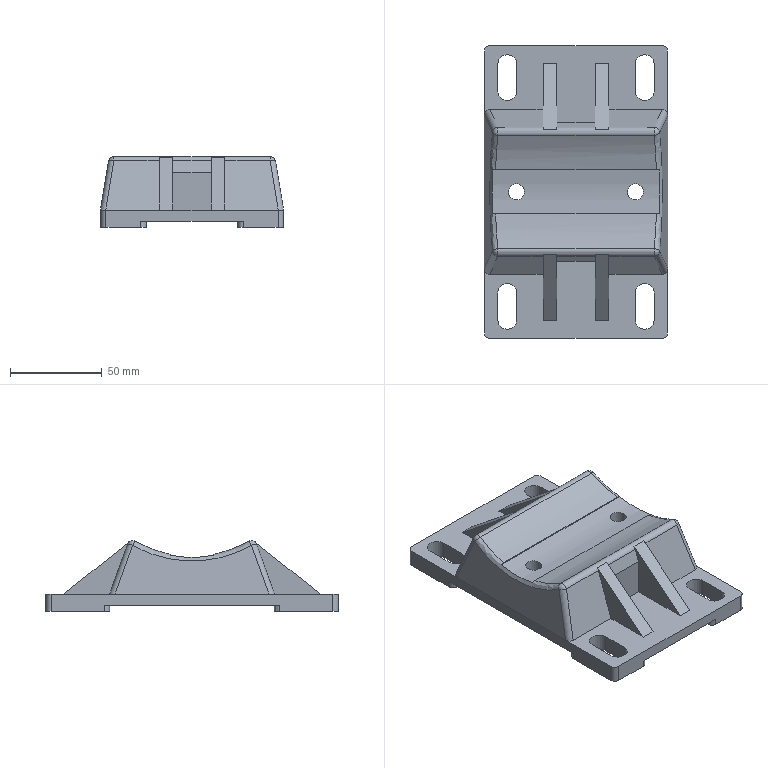Part | STEP file | MDZ Q7A | 1 solid | 121 faces | box 100 x 160 x 38.7 mm | volume 142621 mm3 | plane 75 | cylinder 40 | sphere 4 | spline 2 | commonest cylinder face diameters 6 x22 10.5 x8 8.8 x2 18.8 x2 124 x2 134 x2